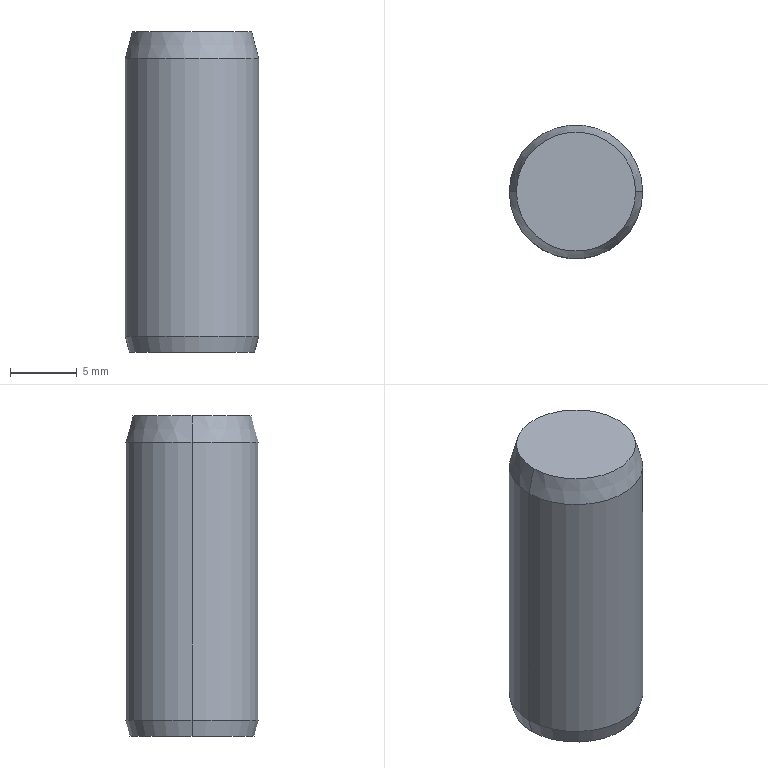Part | SolidWorks | features Chamfer 3, Cut 2, Extrusion 1, RevCut 1 | 1 solid | 16 faces | box 10 x 10 x 24 mm | volume 1497 mm3 | cone 8 | cylinder 6 | plane 2 | commonest cylinder face diameters 5.196 x2 6.4 x2 10 x2
STEP:
#1=CARTESIAN_POINT('',(2.598,0.,1.802));
#2=VERTEX_POINT('',#1);
#3=CARTESIAN_POINT('',(-2.598,0.,1.802));
#4=VERTEX_POINT('',#3);
#5=CARTESIAN_POINT('',(0.,0.,1.802));
#6=DIRECTION('',(0.,0.,-1.));
#7=DIRECTION('',(-1.,0.,0.));
#8=AXIS2_PLACEMENT_3D('',#5,#6,#7);
#9=CIRCLE('',#8,2.598);
#10=EDGE_CURVE('',#2,#4,#9,.T.);
#11=ORIENTED_EDGE('',*,*,#10,.F.);
#12=CARTESIAN_POINT('',(3.2,0.,1.2));
#13=VERTEX_POINT('',#12);
#14=CARTESIAN_POINT('',(3.2,0.,1.2));
#15=DIRECTION('',(0.7071,0.,-0.7071));
#16=VECTOR('',#15,1000.);
#17=LINE('',#14,#16);
#18=EDGE_CURVE('',#2,#13,#17,.T.);
#19=ORIENTED_EDGE('',*,*,#18,.T.);
#20=CARTESIAN_POINT('',(-3.2,0.,1.2));
#21=VERTEX_POINT('',#20);
#22=CARTESIAN_POINT('',(0.,0.,1.2));
#23=DIRECTION('',(0.,0.,-1.));
#24=DIRECTION('',(-1.,0.,0.));
#25=AXIS2_PLACEMENT_3D('',#22,#23,#24);
#26=CIRCLE('',#25,3.2);
#27=EDGE_CURVE('',#13,#21,#26,.T.);
#28=ORIENTED_EDGE('',*,*,#27,.T.);
#29=CARTESIAN_POINT('',(-3.2,0.,1.2));
#30=DIRECTION('',(-0.7071,0.,-0.7071));
#31=VECTOR('',#30,1000.);
#32=LINE('',#29,#31);
#33=EDGE_CURVE('',#4,#21,#32,.T.);
#34=ORIENTED_EDGE('',*,*,#33,.F.);
#35=EDGE_LOOP('',(#11,#19,#28,#34));
#36=FACE_OUTER_BOUND('',#35,.T.);
#37=CARTESIAN_POINT('',(0.,0.,1.2));
#38=DIRECTION('',(0.,0.,-1.));
#39=DIRECTION('',(-1.,0.,0.));
#40=AXIS2_PLACEMENT_3D('',#37,#38,#39);
#41=CONICAL_SURFACE('',#40,3.2,0.7854);
#42=ADVANCED_FACE('',(#36),#41,.F.);
#43=CARTESIAN_POINT('',(-2.598,0.,16.));
#44=VERTEX_POINT('',#43);
#45=CARTESIAN_POINT('',(2.598,0.,16.));
#46=VERTEX_POINT('',#45);
#47=CARTESIAN_POINT('',(0.,0.,16.));
#48=DIRECTION('',(0.,0.,1.));
#49=DIRECTION('',(1.,0.,0.));
#50=AXIS2_PLACEMENT_3D('',#47,#48,#49);
#51=CIRCLE('',#50,2.598);
#52=EDGE_CURVE('',#44,#46,#51,.T.);
#53=ORIENTED_EDGE('',*,*,#52,.T.);
#54=CARTESIAN_POINT('',(2.598,0.,16.));
#55=DIRECTION('',(0.,0.,-1.));
#56=VECTOR('',#55,1000.);
#57=LINE('',#54,#56);
#58=EDGE_CURVE('',#46,#2,#57,.T.);
#59=ORIENTED_EDGE('',*,*,#58,.T.);
#60=ORIENTED_EDGE('',*,*,#10,.T.);
#61=CARTESIAN_POINT('',(-2.598,0.,16.));
#62=DIRECTION('',(0.,0.,-1.));
#63=VECTOR('',#62,1000.);
#64=LINE('',#61,#63);
#65=EDGE_CURVE('',#44,#4,#64,.T.);
#66=ORIENTED_EDGE('',*,*,#65,.F.);
#67=EDGE_LOOP('',(#53,#59,#60,#66));
#68=FACE_OUTER_BOUND('',#67,.T.);
#69=CARTESIAN_POINT('',(0.,0.,16.));
#70=DIRECTION('',(0.,0.,-1.));
#71=DIRECTION('',(-1.,0.,0.));
#72=AXIS2_PLACEMENT_3D('',#69,#70,#71);
#73=CYLINDRICAL_SURFACE('',#72,2.598);
#74=ADVANCED_FACE('',(#68),#73,.F.);
#75=CARTESIAN_POINT('',(0.,0.,17.5));
#76=VERTEX_POINT('',#75);
#77=CARTESIAN_POINT('',(-2.598,0.,16.));
#78=DIRECTION('',(-0.866,0.,-0.5));
#79=VECTOR('',#78,1000.);
#80=LINE('',#77,#79);
#81=EDGE_CURVE('',#76,#44,#80,.T.);
#82=ORIENTED_EDGE('',*,*,#81,.F.);
#83=CARTESIAN_POINT('',(2.598,0.,16.));
#84=DIRECTION('',(0.866,0.,-0.5));
#85=VECTOR('',#84,1000.);
#86=LINE('',#83,#85);
#87=EDGE_CURVE('',#76,#46,#86,.T.);
#88=ORIENTED_EDGE('',*,*,#87,.T.);
#89=ORIENTED_EDGE('',*,*,#52,.F.);
#90=EDGE_LOOP('',(#82,#88,#89));
#91=FACE_OUTER_BOUND('',#90,.T.);
#92=CARTESIAN_POINT('',(0.,0.,16.));
#93=DIRECTION('',(0.,0.,-1.));
#94=DIRECTION('',(-1.,0.,0.));
#95=AXIS2_PLACEMENT_3D('',#92,#93,#94);
#96=CONICAL_SURFACE('',#95,2.598,1.047);
#97=ADVANCED_FACE('',(#91),#96,.F.);
#98=ORIENTED_EDGE('',*,*,#27,.F.);
#99=CARTESIAN_POINT('',(3.2,0.,0.));
#100=VERTEX_POINT('',#99);
#101=CARTESIAN_POINT('',(3.2,0.,1.2));
#102=DIRECTION('',(0.,0.,-1.));
#103=VECTOR('',#102,1000.);
#104=LINE('',#101,#103);
#105=EDGE_CURVE('',#13,#100,#104,.T.);
#106=ORIENTED_EDGE('',*,*,#105,.T.);
#107=CARTESIAN_POINT('',(-3.2,0.,0.));
#108=VERTEX_POINT('',#107);
#109=CARTESIAN_POINT('',(0.,0.,0.));
#110=DIRECTION('',(0.,0.,-1.));
#111=DIRECTION('',(-1.,0.,0.));
#112=AXIS2_PLACEMENT_3D('',#109,#110,#111);
#113=CIRCLE('',#112,3.2);
#114=EDGE_CURVE('',#100,#108,#113,.T.);
#115=ORIENTED_EDGE('',*,*,#114,.T.);
#116=CARTESIAN_POINT('',(-3.2,0.,1.2));
#117=DIRECTION('',(0.,0.,-1.));
#118=VECTOR('',#117,1000.);
#119=LINE('',#116,#118);
#120=EDGE_CURVE('',#21,#108,#119,.T.);
#121=ORIENTED_EDGE('',*,*,#120,.F.);
#122=EDGE_LOOP('',(#98,#106,#115,#121));
#123=FACE_OUTER_BOUND('',#122,.T.);
#124=CARTESIAN_POINT('',(0.,0.,1.2));
#125=DIRECTION('',(0.,0.,-1.));
#126=DIRECTION('',(-1.,0.,0.));
#127=AXIS2_PLACEMENT_3D('',#124,#125,#126);
#128=CYLINDRICAL_SURFACE('',#127,3.2);
#129=ADVANCED_FACE('',(#123),#128,.F.);
#130=CARTESIAN_POINT('',(-4.678,0.,0.));
#131=VERTEX_POINT('',#130);
#132=CARTESIAN_POINT('',(4.678,0.,0.));
#133=VERTEX_POINT('',#132);
#134=CARTESIAN_POINT('',(0.,0.,0.));
#135=DIRECTION('',(0.,0.,-1.));
#136=DIRECTION('',(1.,0.,0.));
#137=AXIS2_PLACEMENT_3D('',#134,#135,#136);
#138=CIRCLE('',#137,4.678);
#139=EDGE_CURVE('',#131,#133,#138,.T.);
#140=ORIENTED_EDGE('',*,*,#139,.F.);
#141=CARTESIAN_POINT('',(-5.,0.,1.2));
#142=VERTEX_POINT('',#141);
#143=CARTESIAN_POINT('',(-5.,0.,1.2));
#144=DIRECTION('',(-0.2588,0.,0.9659));
#145=VECTOR('',#144,1000.);
#146=LINE('',#143,#145);
#147=EDGE_CURVE('',#131,#142,#146,.T.);
#148=ORIENTED_EDGE('',*,*,#147,.T.);
#149=CARTESIAN_POINT('',(5.,0.,1.2));
#150=VERTEX_POINT('',#149);
#151=CARTESIAN_POINT('',(0.,0.,1.2));
#152=DIRECTION('',(0.,0.,1.));
#153=DIRECTION('',(1.,0.,0.));
#154=AXIS2_PLACEMENT_3D('',#151,#152,#153);
#155=CIRCLE('',#154,5.);
#156=EDGE_CURVE('',#150,#142,#155,.T.);
#157=ORIENTED_EDGE('',*,*,#156,.F.);
#158=CARTESIAN_POINT('',(5.,0.,1.2));
#159=DIRECTION('',(0.2588,0.,0.9659));
#160=VECTOR('',#159,1000.);
#161=LINE('',#158,#160);
#162=EDGE_CURVE('',#133,#150,#161,.T.);
#163=ORIENTED_EDGE('',*,*,#162,.F.);
#164=EDGE_LOOP('',(#140,#148,#157,#163));
#165=FACE_OUTER_BOUND('',#164,.T.);
#166=CARTESIAN_POINT('',(0.,0.,1.2));
#167=DIRECTION('',(0.,0.,1.));
#168=DIRECTION('',(1.,0.,0.));
#169=AXIS2_PLACEMENT_3D('',#166,#167,#168);
#170=CONICAL_SURFACE('',#169,5.,0.2618);
#171=ADVANCED_FACE('',(#165),#170,.T.);
#172=CARTESIAN_POINT('',(4.464,0.,24.));
#173=VERTEX_POINT('',#172);
#174=CARTESIAN_POINT('',(-4.464,0.,24.));
#175=VERTEX_POINT('',#174);
#176=CARTESIAN_POINT('',(0.,0.,24.));
#177=DIRECTION('',(0.,0.,1.));
#178=DIRECTION('',(1.,0.,0.));
#179=AXIS2_PLACEMENT_3D('',#176,#177,#178);
#180=CIRCLE('',#179,4.464);
#181=EDGE_CURVE('',#173,#175,#180,.T.);
#182=ORIENTED_EDGE('',*,*,#181,.F.);
#183=CARTESIAN_POINT('',(5.,0.,22.));
#184=VERTEX_POINT('',#183);
#185=CARTESIAN_POINT('',(4.464,0.,24.));
#186=DIRECTION('',(0.2588,0.,-0.9659));
#187=VECTOR('',#186,1000.);
#188=LINE('',#185,#187);
#189=EDGE_CURVE('',#173,#184,#188,.T.);
#190=ORIENTED_EDGE('',*,*,#189,.T.);
#191=CARTESIAN_POINT('',(-5.,0.,22.));
#192=VERTEX_POINT('',#191);
#193=CARTESIAN_POINT('',(0.,0.,22.));
#194=DIRECTION('',(0.,0.,-1.));
#195=DIRECTION('',(1.,0.,0.));
#196=AXIS2_PLACEMENT_3D('',#193,#194,#195);
#197=CIRCLE('',#196,5.);
#198=EDGE_CURVE('',#192,#184,#197,.T.);
#199=ORIENTED_EDGE('',*,*,#198,.F.);
#200=CARTESIAN_POINT('',(-4.464,0.,24.));
#201=DIRECTION('',(-0.2588,0.,-0.9659));
#202=VECTOR('',#201,1000.);
#203=LINE('',#200,#202);
#204=EDGE_CURVE('',#175,#192,#203,.T.);
#205=ORIENTED_EDGE('',*,*,#204,.F.);
#206=EDGE_LOOP('',(#182,#190,#199,#205));
#207=FACE_OUTER_BOUND('',#206,.T.);
#208=CARTESIAN_POINT('',(0.,0.,24.));
#209=DIRECTION('',(0.,0.,-1.));
#210=DIRECTION('',(-1.,0.,0.));
#211=AXIS2_PLACEMENT_3D('',#208,#209,#210);
#212=CONICAL_SURFACE('',#211,4.464,0.2618);
#213=ADVANCED_FACE('',(#207),#212,.T.);
#214=ORIENTED_EDGE('',*,*,#198,.T.);
#215=CARTESIAN_POINT('',(5.,0.,24.));
#216=DIRECTION('',(0.,0.,-1.));
#217=VECTOR('',#216,1000.);
#218=LINE('',#215,#217);
#219=EDGE_CURVE('',#184,#150,#218,.T.);
#220=ORIENTED_EDGE('',*,*,#219,.T.);
#221=ORIENTED_EDGE('',*,*,#156,.T.);
#222=CARTESIAN_POINT('',(-5.,0.,24.));
#223=DIRECTION('',(0.,0.,-1.));
#224=VECTOR('',#223,1000.);
#225=LINE('',#222,#224);
#226=EDGE_CURVE('',#192,#142,#225,.T.);
#227=ORIENTED_EDGE('',*,*,#226,.F.);
#228=EDGE_LOOP('',(#214,#220,#221,#227));
#229=FACE_OUTER_BOUND('',#228,.T.);
#230=CARTESIAN_POINT('',(0.,0.,24.));
#231=DIRECTION('',(0.,0.,-1.));
#232=DIRECTION('',(-1.,0.,0.));
#233=AXIS2_PLACEMENT_3D('',#230,#231,#232);
#234=CYLINDRICAL_SURFACE('',#233,5.);
#235=ADVANCED_FACE('',(#229),#234,.T.);
#236=ORIENTED_EDGE('',*,*,#219,.F.);
#237=CARTESIAN_POINT('',(0.,0.,22.));
#238=DIRECTION('',(0.,0.,-1.));
#239=DIRECTION('',(1.,0.,0.));
#240=AXIS2_PLACEMENT_3D('',#237,#238,#239);
#241=CIRCLE('',#240,5.);
#242=EDGE_CURVE('',#184,#192,#241,.T.);
#243=ORIENTED_EDGE('',*,*,#242,.T.);
#244=ORIENTED_EDGE('',*,*,#226,.T.);
#245=CARTESIAN_POINT('',(0.,0.,1.2));
#246=DIRECTION('',(0.,0.,1.));
#247=DIRECTION('',(1.,0.,0.));
#248=AXIS2_PLACEMENT_3D('',#245,#246,#247);
#249=CIRCLE('',#248,5.);
#250=EDGE_CURVE('',#142,#150,#249,.T.);
#251=ORIENTED_EDGE('',*,*,#250,.T.);
#252=EDGE_LOOP('',(#236,#243,#244,#251));
#253=FACE_OUTER_BOUND('',#252,.T.);
#254=CARTESIAN_POINT('',(0.,0.,24.));
#255=DIRECTION('',(0.,0.,-1.));
#256=DIRECTION('',(-1.,0.,0.));
#257=AXIS2_PLACEMENT_3D('',#254,#255,#256);
#258=CYLINDRICAL_SURFACE('',#257,5.);
#259=ADVANCED_FACE('',(#253),#258,.T.);
#260=CARTESIAN_POINT('',(0.,0.,24.));
#261=DIRECTION('',(0.,0.,1.));
#262=DIRECTION('',(1.,0.,0.));
#263=AXIS2_PLACEMENT_3D('',#260,#261,#262);
#264=CIRCLE('',#263,4.464);
#265=EDGE_CURVE('',#175,#173,#264,.T.);
#266=ORIENTED_EDGE('',*,*,#265,.T.);
#267=ORIENTED_EDGE('',*,*,#181,.T.);
#268=EDGE_LOOP('',(#266,#267));
#269=FACE_OUTER_BOUND('',#268,.T.);
#270=CARTESIAN_POINT('',(0.,0.,24.));
#271=DIRECTION('',(0.,0.,1.));
#272=DIRECTION('',(1.,0.,0.));
#273=AXIS2_PLACEMENT_3D('',#270,#271,#272);
#274=PLANE('',#273);
#275=ADVANCED_FACE('',(#269),#274,.T.);
#276=CARTESIAN_POINT('',(0.,0.,0.));
#277=DIRECTION('',(0.,0.,-1.));
#278=DIRECTION('',(-1.,0.,0.));
#279=AXIS2_PLACEMENT_3D('',#276,#277,#278);
#280=CIRCLE('',#279,3.2);
#281=EDGE_CURVE('',#108,#100,#280,.T.);
#282=ORIENTED_EDGE('',*,*,#281,.F.);
#283=ORIENTED_EDGE('',*,*,#114,.F.);
#284=EDGE_LOOP('',(#282,#283));
#285=FACE_BOUND('',#284,.T.);
#286=CARTESIAN_POINT('',(0.,0.,0.));
#287=DIRECTION('',(0.,0.,-1.));
#288=DIRECTION('',(1.,0.,0.));
#289=AXIS2_PLACEMENT_3D('',#286,#287,#288);
#290=CIRCLE('',#289,4.678);
#291=EDGE_CURVE('',#133,#131,#290,.T.);
#292=ORIENTED_EDGE('',*,*,#291,.T.);
#293=ORIENTED_EDGE('',*,*,#139,.T.);
#294=EDGE_LOOP('',(#292,#293));
#295=FACE_OUTER_BOUND('',#294,.T.);
#296=CARTESIAN_POINT('',(0.,0.,0.));
#297=DIRECTION('',(0.,0.,1.));
#298=DIRECTION('',(1.,0.,0.));
#299=AXIS2_PLACEMENT_3D('',#296,#297,#298);
#300=PLANE('',#299);
#301=ADVANCED_FACE('',(#285,#295),#300,.F.);
#302=ORIENTED_EDGE('',*,*,#189,.F.);
#303=ORIENTED_EDGE('',*,*,#265,.F.);
#304=ORIENTED_EDGE('',*,*,#204,.T.);
#305=ORIENTED_EDGE('',*,*,#242,.F.);
#306=EDGE_LOOP('',(#302,#303,#304,#305));
#307=FACE_OUTER_BOUND('',#306,.T.);
#308=CARTESIAN_POINT('',(0.,0.,24.));
#309=DIRECTION('',(0.,0.,-1.));
#310=DIRECTION('',(-1.,0.,0.));
#311=AXIS2_PLACEMENT_3D('',#308,#309,#310);
#312=CONICAL_SURFACE('',#311,4.464,0.2618);
#313=ADVANCED_FACE('',(#307),#312,.T.);
#314=ORIENTED_EDGE('',*,*,#147,.F.);
#315=ORIENTED_EDGE('',*,*,#291,.F.);
#316=ORIENTED_EDGE('',*,*,#162,.T.);
#317=ORIENTED_EDGE('',*,*,#250,.F.);
#318=EDGE_LOOP('',(#314,#315,#316,#317));
#319=FACE_OUTER_BOUND('',#318,.T.);
#320=CARTESIAN_POINT('',(0.,0.,1.2));
#321=DIRECTION('',(0.,0.,1.));
#322=DIRECTION('',(1.,0.,0.));
#323=AXIS2_PLACEMENT_3D('',#320,#321,#322);
#324=CONICAL_SURFACE('',#323,5.,0.2618);
#325=ADVANCED_FACE('',(#319),#324,.T.);
#326=ORIENTED_EDGE('',*,*,#105,.F.);
#327=CARTESIAN_POINT('',(0.,0.,1.2));
#328=DIRECTION('',(0.,0.,-1.));
#329=DIRECTION('',(-1.,0.,0.));
#330=AXIS2_PLACEMENT_3D('',#327,#328,#329);
#331=CIRCLE('',#330,3.2);
#332=EDGE_CURVE('',#21,#13,#331,.T.);
#333=ORIENTED_EDGE('',*,*,#332,.F.);
#334=ORIENTED_EDGE('',*,*,#120,.T.);
#335=ORIENTED_EDGE('',*,*,#281,.T.);
#336=EDGE_LOOP('',(#326,#333,#334,#335));
#337=FACE_OUTER_BOUND('',#336,.T.);
#338=CARTESIAN_POINT('',(0.,0.,1.2));
#339=DIRECTION('',(0.,0.,-1.));
#340=DIRECTION('',(-1.,0.,0.));
#341=AXIS2_PLACEMENT_3D('',#338,#339,#340);
#342=CYLINDRICAL_SURFACE('',#341,3.2);
#343=ADVANCED_FACE('',(#337),#342,.F.);
#344=ORIENTED_EDGE('',*,*,#87,.F.);
#345=ORIENTED_EDGE('',*,*,#81,.T.);
#346=CARTESIAN_POINT('',(0.,0.,16.));
#347=DIRECTION('',(0.,0.,1.));
#348=DIRECTION('',(1.,0.,0.));
#349=AXIS2_PLACEMENT_3D('',#346,#347,#348);
#350=CIRCLE('',#349,2.598);
#351=EDGE_CURVE('',#46,#44,#350,.T.);
#352=ORIENTED_EDGE('',*,*,#351,.F.);
#353=EDGE_LOOP('',(#344,#345,#352));
#354=FACE_OUTER_BOUND('',#353,.T.);
#355=CARTESIAN_POINT('',(0.,0.,16.));
#356=DIRECTION('',(0.,0.,-1.));
#357=DIRECTION('',(-1.,0.,0.));
#358=AXIS2_PLACEMENT_3D('',#355,#356,#357);
#359=CONICAL_SURFACE('',#358,2.598,1.047);
#360=ADVANCED_FACE('',(#354),#359,.F.);
#361=ORIENTED_EDGE('',*,*,#58,.F.);
#362=ORIENTED_EDGE('',*,*,#351,.T.);
#363=ORIENTED_EDGE('',*,*,#65,.T.);
#364=CARTESIAN_POINT('',(0.,0.,1.802));
#365=DIRECTION('',(0.,0.,-1.));
#366=DIRECTION('',(-1.,0.,0.));
#367=AXIS2_PLACEMENT_3D('',#364,#365,#366);
#368=CIRCLE('',#367,2.598);
#369=EDGE_CURVE('',#4,#2,#368,.T.);
#370=ORIENTED_EDGE('',*,*,#369,.T.);
#371=EDGE_LOOP('',(#361,#362,#363,#370));
#372=FACE_OUTER_BOUND('',#371,.T.);
#373=CARTESIAN_POINT('',(0.,0.,16.));
#374=DIRECTION('',(0.,0.,-1.));
#375=DIRECTION('',(-1.,0.,0.));
#376=AXIS2_PLACEMENT_3D('',#373,#374,#375);
#377=CYLINDRICAL_SURFACE('',#376,2.598);
#378=ADVANCED_FACE('',(#372),#377,.F.);
#379=ORIENTED_EDGE('',*,*,#18,.F.);
#380=ORIENTED_EDGE('',*,*,#369,.F.);
#381=ORIENTED_EDGE('',*,*,#33,.T.);
#382=ORIENTED_EDGE('',*,*,#332,.T.);
#383=EDGE_LOOP('',(#379,#380,#381,#382));
#384=FACE_OUTER_BOUND('',#383,.T.);
#385=CARTESIAN_POINT('',(0.,0.,1.2));
#386=DIRECTION('',(0.,0.,-1.));
#387=DIRECTION('',(-1.,0.,0.));
#388=AXIS2_PLACEMENT_3D('',#385,#386,#387);
#389=CONICAL_SURFACE('',#388,3.2,0.7854);
#390=ADVANCED_FACE('',(#384),#389,.F.);
#391=CLOSED_SHELL('',(#42,#74,#97,#129,#171,#213,#235,#259,#275,#301,#313,#325,#343,#360,#378,#390));
#392=MANIFOLD_SOLID_BREP('',#391);
#393=CARTESIAN_POINT('',(0.,0.,0.));
#394=DIRECTION('',(0.,0.,1.));
#395=DIRECTION('',(1.,0.,0.));
#396=AXIS2_PLACEMENT_3D('',#393,#394,#395);
#397=(LENGTH_UNIT()NAMED_UNIT(*)SI_UNIT(.MILLI.,.METRE.));
#398=UNCERTAINTY_MEASURE_WITH_UNIT(LENGTH_MEASURE(0.00001),#397,'','');
#399=(NAMED_UNIT(*)PLANE_ANGLE_UNIT()SI_UNIT($,.RADIAN.));
#400=(NAMED_UNIT(*)SI_UNIT($,.STERADIAN.)SOLID_ANGLE_UNIT());
#401=(GEOMETRIC_REPRESENTATION_CONTEXT(3)GLOBAL_UNCERTAINTY_ASSIGNED_CONTEXT((#398))GLOBAL_UNIT_ASSIGNED_CONTEXT((#397,#399,#400))REPRESENTATION_CONTEXT('',''));
#402=ADVANCED_BREP_SHAPE_REPRESENTATION('',(#392,#396),#401);